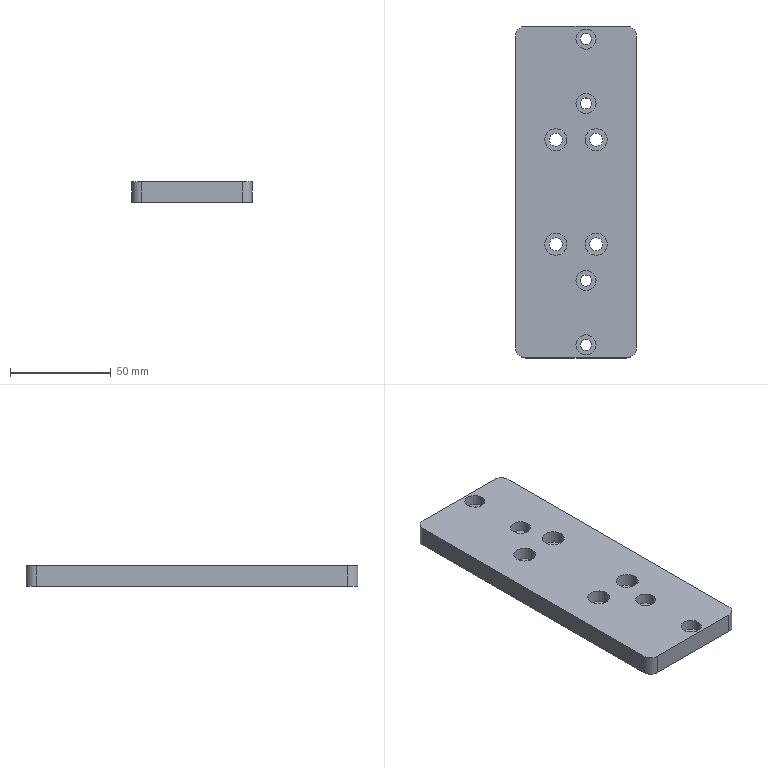Part | SolidWorks | features HoleWzd 2, Extrusion 1, Fillet 1 | 1 solid | 50 faces | box 60 x 165 x 10 mm | volume 93726 mm3 | cylinder 36 | plane 14 | commonest cylinder face diameters 10 x12 5.5 x8 6.6 x8 11 x8
STEP:
#1=CARTESIAN_POINT('',(-0.05704,76.,4.6));
#2=VERTEX_POINT('',#1);
#3=CARTESIAN_POINT('',(9.943,76.,4.6));
#4=VERTEX_POINT('',#3);
#5=CARTESIAN_POINT('',(4.943,76.,4.6));
#6=DIRECTION('',(0.,0.,1.));
#7=DIRECTION('',(1.,0.,0.));
#8=AXIS2_PLACEMENT_3D('',#5,#6,#7);
#9=CIRCLE('',#8,5.);
#10=EDGE_CURVE('',#2,#4,#9,.T.);
#11=ORIENTED_EDGE('',*,*,#10,.F.);
#12=CARTESIAN_POINT('',(-0.05704,76.,10.));
#13=VERTEX_POINT('',#12);
#14=CARTESIAN_POINT('',(-0.05704,76.,10.));
#15=DIRECTION('',(0.,0.,1.));
#16=VECTOR('',#15,1000.);
#17=LINE('',#14,#16);
#18=EDGE_CURVE('',#2,#13,#17,.T.);
#19=ORIENTED_EDGE('',*,*,#18,.T.);
#20=CARTESIAN_POINT('',(9.943,76.,10.));
#21=VERTEX_POINT('',#20);
#22=CARTESIAN_POINT('',(4.943,76.,10.));
#23=DIRECTION('',(0.,0.,1.));
#24=DIRECTION('',(1.,0.,0.));
#25=AXIS2_PLACEMENT_3D('',#22,#23,#24);
#26=CIRCLE('',#25,5.);
#27=EDGE_CURVE('',#13,#21,#26,.T.);
#28=ORIENTED_EDGE('',*,*,#27,.T.);
#29=CARTESIAN_POINT('',(9.943,76.,10.));
#30=DIRECTION('',(0.,0.,1.));
#31=VECTOR('',#30,1000.);
#32=LINE('',#29,#31);
#33=EDGE_CURVE('',#4,#21,#32,.T.);
#34=ORIENTED_EDGE('',*,*,#33,.F.);
#35=EDGE_LOOP('',(#11,#19,#28,#34));
#36=FACE_OUTER_BOUND('',#35,.T.);
#37=CARTESIAN_POINT('',(4.943,76.,10.));
#38=DIRECTION('',(0.,0.,1.));
#39=DIRECTION('',(1.,0.,0.));
#40=AXIS2_PLACEMENT_3D('',#37,#38,#39);
#41=CYLINDRICAL_SURFACE('',#40,5.);
#42=ADVANCED_FACE('',(#36),#41,.F.);
#43=CARTESIAN_POINT('',(2.193,76.,0.));
#44=VERTEX_POINT('',#43);
#45=CARTESIAN_POINT('',(7.693,76.,0.));
#46=VERTEX_POINT('',#45);
#47=CARTESIAN_POINT('',(4.943,76.,0.));
#48=DIRECTION('',(0.,0.,1.));
#49=DIRECTION('',(1.,0.,0.));
#50=AXIS2_PLACEMENT_3D('',#47,#48,#49);
#51=CIRCLE('',#50,2.75);
#52=EDGE_CURVE('',#44,#46,#51,.T.);
#53=ORIENTED_EDGE('',*,*,#52,.F.);
#54=CARTESIAN_POINT('',(2.193,76.,4.6));
#55=VERTEX_POINT('',#54);
#56=CARTESIAN_POINT('',(2.193,76.,10.));
#57=DIRECTION('',(0.,0.,1.));
#58=VECTOR('',#57,1000.);
#59=LINE('',#56,#58);
#60=EDGE_CURVE('',#44,#55,#59,.T.);
#61=ORIENTED_EDGE('',*,*,#60,.T.);
#62=CARTESIAN_POINT('',(7.693,76.,4.6));
#63=VERTEX_POINT('',#62);
#64=CARTESIAN_POINT('',(4.943,76.,4.6));
#65=DIRECTION('',(0.,0.,1.));
#66=DIRECTION('',(1.,0.,0.));
#67=AXIS2_PLACEMENT_3D('',#64,#65,#66);
#68=CIRCLE('',#67,2.75);
#69=EDGE_CURVE('',#55,#63,#68,.T.);
#70=ORIENTED_EDGE('',*,*,#69,.T.);
#71=CARTESIAN_POINT('',(7.693,76.,10.));
#72=DIRECTION('',(0.,0.,1.));
#73=VECTOR('',#72,1000.);
#74=LINE('',#71,#73);
#75=EDGE_CURVE('',#46,#63,#74,.T.);
#76=ORIENTED_EDGE('',*,*,#75,.F.);
#77=EDGE_LOOP('',(#53,#61,#70,#76));
#78=FACE_OUTER_BOUND('',#77,.T.);
#79=CARTESIAN_POINT('',(4.943,76.,10.));
#80=DIRECTION('',(0.,0.,1.));
#81=DIRECTION('',(1.,0.,0.));
#82=AXIS2_PLACEMENT_3D('',#79,#80,#81);
#83=CYLINDRICAL_SURFACE('',#82,2.75);
#84=ADVANCED_FACE('',(#78),#83,.F.);
#85=CARTESIAN_POINT('',(-0.05704,44.,4.6));
#86=VERTEX_POINT('',#85);
#87=CARTESIAN_POINT('',(9.943,44.,4.6));
#88=VERTEX_POINT('',#87);
#89=CARTESIAN_POINT('',(4.943,44.,4.6));
#90=DIRECTION('',(0.,0.,1.));
#91=DIRECTION('',(1.,0.,0.));
#92=AXIS2_PLACEMENT_3D('',#89,#90,#91);
#93=CIRCLE('',#92,5.);
#94=EDGE_CURVE('',#86,#88,#93,.T.);
#95=ORIENTED_EDGE('',*,*,#94,.F.);
#96=CARTESIAN_POINT('',(-0.05704,44.,10.));
#97=VERTEX_POINT('',#96);
#98=CARTESIAN_POINT('',(-0.05704,44.,10.));
#99=DIRECTION('',(0.,0.,1.));
#100=VECTOR('',#99,1000.);
#101=LINE('',#98,#100);
#102=EDGE_CURVE('',#86,#97,#101,.T.);
#103=ORIENTED_EDGE('',*,*,#102,.T.);
#104=CARTESIAN_POINT('',(9.943,44.,10.));
#105=VERTEX_POINT('',#104);
#106=CARTESIAN_POINT('',(4.943,44.,10.));
#107=DIRECTION('',(0.,0.,1.));
#108=DIRECTION('',(1.,0.,0.));
#109=AXIS2_PLACEMENT_3D('',#106,#107,#108);
#110=CIRCLE('',#109,5.);
#111=EDGE_CURVE('',#97,#105,#110,.T.);
#112=ORIENTED_EDGE('',*,*,#111,.T.);
#113=CARTESIAN_POINT('',(9.943,44.,10.));
#114=DIRECTION('',(0.,0.,1.));
#115=VECTOR('',#114,1000.);
#116=LINE('',#113,#115);
#117=EDGE_CURVE('',#88,#105,#116,.T.);
#118=ORIENTED_EDGE('',*,*,#117,.F.);
#119=EDGE_LOOP('',(#95,#103,#112,#118));
#120=FACE_OUTER_BOUND('',#119,.T.);
#121=CARTESIAN_POINT('',(4.943,44.,10.));
#122=DIRECTION('',(0.,0.,1.));
#123=DIRECTION('',(1.,0.,0.));
#124=AXIS2_PLACEMENT_3D('',#121,#122,#123);
#125=CYLINDRICAL_SURFACE('',#124,5.);
#126=ADVANCED_FACE('',(#120),#125,.F.);
#127=CARTESIAN_POINT('',(2.193,44.,0.));
#128=VERTEX_POINT('',#127);
#129=CARTESIAN_POINT('',(7.693,44.,0.));
#130=VERTEX_POINT('',#129);
#131=CARTESIAN_POINT('',(4.943,44.,0.));
#132=DIRECTION('',(0.,0.,1.));
#133=DIRECTION('',(1.,0.,0.));
#134=AXIS2_PLACEMENT_3D('',#131,#132,#133);
#135=CIRCLE('',#134,2.75);
#136=EDGE_CURVE('',#128,#130,#135,.T.);
#137=ORIENTED_EDGE('',*,*,#136,.F.);
#138=CARTESIAN_POINT('',(2.193,44.,4.6));
#139=VERTEX_POINT('',#138);
#140=CARTESIAN_POINT('',(2.193,44.,10.));
#141=DIRECTION('',(0.,0.,1.));
#142=VECTOR('',#141,1000.);
#143=LINE('',#140,#142);
#144=EDGE_CURVE('',#128,#139,#143,.T.);
#145=ORIENTED_EDGE('',*,*,#144,.T.);
#146=CARTESIAN_POINT('',(7.693,44.,4.6));
#147=VERTEX_POINT('',#146);
#148=CARTESIAN_POINT('',(4.943,44.,4.6));
#149=DIRECTION('',(0.,0.,1.));
#150=DIRECTION('',(1.,0.,0.));
#151=AXIS2_PLACEMENT_3D('',#148,#149,#150);
#152=CIRCLE('',#151,2.75);
#153=EDGE_CURVE('',#139,#147,#152,.T.);
#154=ORIENTED_EDGE('',*,*,#153,.T.);
#155=CARTESIAN_POINT('',(7.693,44.,10.));
#156=DIRECTION('',(0.,0.,1.));
#157=VECTOR('',#156,1000.);
#158=LINE('',#155,#157);
#159=EDGE_CURVE('',#130,#147,#158,.T.);
#160=ORIENTED_EDGE('',*,*,#159,.F.);
#161=EDGE_LOOP('',(#137,#145,#154,#160));
#162=FACE_OUTER_BOUND('',#161,.T.);
#163=CARTESIAN_POINT('',(4.943,44.,10.));
#164=DIRECTION('',(0.,0.,1.));
#165=DIRECTION('',(1.,0.,0.));
#166=AXIS2_PLACEMENT_3D('',#163,#164,#165);
#167=CYLINDRICAL_SURFACE('',#166,2.75);
#168=ADVANCED_FACE('',(#162),#167,.F.);
#169=CARTESIAN_POINT('',(-0.05704,-44.,4.6));
#170=VERTEX_POINT('',#169);
#171=CARTESIAN_POINT('',(9.943,-44.,4.6));
#172=VERTEX_POINT('',#171);
#173=CARTESIAN_POINT('',(4.943,-44.,4.6));
#174=DIRECTION('',(0.,0.,1.));
#175=DIRECTION('',(1.,0.,0.));
#176=AXIS2_PLACEMENT_3D('',#173,#174,#175);
#177=CIRCLE('',#176,5.);
#178=EDGE_CURVE('',#170,#172,#177,.T.);
#179=ORIENTED_EDGE('',*,*,#178,.F.);
#180=CARTESIAN_POINT('',(-0.05704,-44.,10.));
#181=VERTEX_POINT('',#180);
#182=CARTESIAN_POINT('',(-0.05704,-44.,10.));
#183=DIRECTION('',(0.,0.,1.));
#184=VECTOR('',#183,1000.);
#185=LINE('',#182,#184);
#186=EDGE_CURVE('',#170,#181,#185,.T.);
#187=ORIENTED_EDGE('',*,*,#186,.T.);
#188=CARTESIAN_POINT('',(9.943,-44.,10.));
#189=VERTEX_POINT('',#188);
#190=CARTESIAN_POINT('',(4.943,-44.,10.));
#191=DIRECTION('',(0.,0.,1.));
#192=DIRECTION('',(1.,0.,0.));
#193=AXIS2_PLACEMENT_3D('',#190,#191,#192);
#194=CIRCLE('',#193,5.);
#195=EDGE_CURVE('',#181,#189,#194,.T.);
#196=ORIENTED_EDGE('',*,*,#195,.T.);
#197=CARTESIAN_POINT('',(9.943,-44.,10.));
#198=DIRECTION('',(0.,0.,1.));
#199=VECTOR('',#198,1000.);
#200=LINE('',#197,#199);
#201=EDGE_CURVE('',#172,#189,#200,.T.);
#202=ORIENTED_EDGE('',*,*,#201,.F.);
#203=EDGE_LOOP('',(#179,#187,#196,#202));
#204=FACE_OUTER_BOUND('',#203,.T.);
#205=CARTESIAN_POINT('',(4.943,-44.,10.));
#206=DIRECTION('',(0.,0.,1.));
#207=DIRECTION('',(1.,0.,0.));
#208=AXIS2_PLACEMENT_3D('',#205,#206,#207);
#209=CYLINDRICAL_SURFACE('',#208,5.);
#210=ADVANCED_FACE('',(#204),#209,.F.);
#211=CARTESIAN_POINT('',(2.193,-44.,0.));
#212=VERTEX_POINT('',#211);
#213=CARTESIAN_POINT('',(7.693,-44.,0.));
#214=VERTEX_POINT('',#213);
#215=CARTESIAN_POINT('',(4.943,-44.,0.));
#216=DIRECTION('',(0.,0.,1.));
#217=DIRECTION('',(1.,0.,0.));
#218=AXIS2_PLACEMENT_3D('',#215,#216,#217);
#219=CIRCLE('',#218,2.75);
#220=EDGE_CURVE('',#212,#214,#219,.T.);
#221=ORIENTED_EDGE('',*,*,#220,.F.);
#222=CARTESIAN_POINT('',(2.193,-44.,4.6));
#223=VERTEX_POINT('',#222);
#224=CARTESIAN_POINT('',(2.193,-44.,10.));
#225=DIRECTION('',(0.,0.,1.));
#226=VECTOR('',#225,1000.);
#227=LINE('',#224,#226);
#228=EDGE_CURVE('',#212,#223,#227,.T.);
#229=ORIENTED_EDGE('',*,*,#228,.T.);
#230=CARTESIAN_POINT('',(7.693,-44.,4.6));
#231=VERTEX_POINT('',#230);
#232=CARTESIAN_POINT('',(4.943,-44.,4.6));
#233=DIRECTION('',(0.,0.,1.));
#234=DIRECTION('',(1.,0.,0.));
#235=AXIS2_PLACEMENT_3D('',#232,#233,#234);
#236=CIRCLE('',#235,2.75);
#237=EDGE_CURVE('',#223,#231,#236,.T.);
#238=ORIENTED_EDGE('',*,*,#237,.T.);
#239=CARTESIAN_POINT('',(7.693,-44.,10.));
#240=DIRECTION('',(0.,0.,1.));
#241=VECTOR('',#240,1000.);
#242=LINE('',#239,#241);
#243=EDGE_CURVE('',#214,#231,#242,.T.);
#244=ORIENTED_EDGE('',*,*,#243,.F.);
#245=EDGE_LOOP('',(#221,#229,#238,#244));
#246=FACE_OUTER_BOUND('',#245,.T.);
#247=CARTESIAN_POINT('',(4.943,-44.,10.));
#248=DIRECTION('',(0.,0.,1.));
#249=DIRECTION('',(1.,0.,0.));
#250=AXIS2_PLACEMENT_3D('',#247,#248,#249);
#251=CYLINDRICAL_SURFACE('',#250,2.75);
#252=ADVANCED_FACE('',(#246),#251,.F.);
#253=CARTESIAN_POINT('',(-0.05704,-76.,4.6));
#254=VERTEX_POINT('',#253);
#255=CARTESIAN_POINT('',(9.943,-76.,4.6));
#256=VERTEX_POINT('',#255);
#257=CARTESIAN_POINT('',(4.943,-76.,4.6));
#258=DIRECTION('',(0.,0.,1.));
#259=DIRECTION('',(1.,0.,0.));
#260=AXIS2_PLACEMENT_3D('',#257,#258,#259);
#261=CIRCLE('',#260,5.);
#262=EDGE_CURVE('',#254,#256,#261,.T.);
#263=ORIENTED_EDGE('',*,*,#262,.F.);
#264=CARTESIAN_POINT('',(-0.05704,-76.,10.));
#265=VERTEX_POINT('',#264);
#266=CARTESIAN_POINT('',(-0.05704,-76.,10.));
#267=DIRECTION('',(0.,0.,1.));
#268=VECTOR('',#267,1000.);
#269=LINE('',#266,#268);
#270=EDGE_CURVE('',#254,#265,#269,.T.);
#271=ORIENTED_EDGE('',*,*,#270,.T.);
#272=CARTESIAN_POINT('',(9.943,-76.,10.));
#273=VERTEX_POINT('',#272);
#274=CARTESIAN_POINT('',(4.943,-76.,10.));
#275=DIRECTION('',(0.,0.,1.));
#276=DIRECTION('',(1.,0.,0.));
#277=AXIS2_PLACEMENT_3D('',#274,#275,#276);
#278=CIRCLE('',#277,5.);
#279=EDGE_CURVE('',#265,#273,#278,.T.);
#280=ORIENTED_EDGE('',*,*,#279,.T.);
#281=CARTESIAN_POINT('',(9.943,-76.,10.));
#282=DIRECTION('',(0.,0.,1.));
#283=VECTOR('',#282,1000.);
#284=LINE('',#281,#283);
#285=EDGE_CURVE('',#256,#273,#284,.T.);
#286=ORIENTED_EDGE('',*,*,#285,.F.);
#287=EDGE_LOOP('',(#263,#271,#280,#286));
#288=FACE_OUTER_BOUND('',#287,.T.);
#289=CARTESIAN_POINT('',(4.943,-76.,10.));
#290=DIRECTION('',(0.,0.,1.));
#291=DIRECTION('',(1.,0.,0.));
#292=AXIS2_PLACEMENT_3D('',#289,#290,#291);
#293=CYLINDRICAL_SURFACE('',#292,5.);
#294=ADVANCED_FACE('',(#288),#293,.F.);
#295=CARTESIAN_POINT('',(2.193,-76.,0.));
#296=VERTEX_POINT('',#295);
#297=CARTESIAN_POINT('',(7.693,-76.,0.));
#298=VERTEX_POINT('',#297);
#299=CARTESIAN_POINT('',(4.943,-76.,0.));
#300=DIRECTION('',(0.,0.,1.));
#301=DIRECTION('',(1.,0.,0.));
#302=AXIS2_PLACEMENT_3D('',#299,#300,#301);
#303=CIRCLE('',#302,2.75);
#304=EDGE_CURVE('',#296,#298,#303,.T.);
#305=ORIENTED_EDGE('',*,*,#304,.F.);
#306=CARTESIAN_POINT('',(2.193,-76.,4.6));
#307=VERTEX_POINT('',#306);
#308=CARTESIAN_POINT('',(2.193,-76.,10.));
#309=DIRECTION('',(0.,0.,1.));
#310=VECTOR('',#309,1000.);
#311=LINE('',#308,#310);
#312=EDGE_CURVE('',#296,#307,#311,.T.);
#313=ORIENTED_EDGE('',*,*,#312,.T.);
#314=CARTESIAN_POINT('',(7.693,-76.,4.6));
#315=VERTEX_POINT('',#314);
#316=CARTESIAN_POINT('',(4.943,-76.,4.6));
#317=DIRECTION('',(0.,0.,1.));
#318=DIRECTION('',(1.,0.,0.));
#319=AXIS2_PLACEMENT_3D('',#316,#317,#318);
#320=CIRCLE('',#319,2.75);
#321=EDGE_CURVE('',#307,#315,#320,.T.);
#322=ORIENTED_EDGE('',*,*,#321,.T.);
#323=CARTESIAN_POINT('',(7.693,-76.,10.));
#324=DIRECTION('',(0.,0.,1.));
#325=VECTOR('',#324,1000.);
#326=LINE('',#323,#325);
#327=EDGE_CURVE('',#298,#315,#326,.T.);
#328=ORIENTED_EDGE('',*,*,#327,.F.);
#329=EDGE_LOOP('',(#305,#313,#322,#328));
#330=FACE_OUTER_BOUND('',#329,.T.);
#331=CARTESIAN_POINT('',(4.943,-76.,10.));
#332=DIRECTION('',(0.,0.,1.));
#333=DIRECTION('',(1.,0.,0.));
#334=AXIS2_PLACEMENT_3D('',#331,#332,#333);
#335=CYLINDRICAL_SURFACE('',#334,2.75);
#336=ADVANCED_FACE('',(#330),#335,.F.);
#337=CARTESIAN_POINT('',(-15.5,26.,3.6));
#338=VERTEX_POINT('',#337);
#339=CARTESIAN_POINT('',(-4.5,26.,3.6));
#340=VERTEX_POINT('',#339);
#341=CARTESIAN_POINT('',(-10.,26.,3.6));
#342=DIRECTION('',(0.,0.,1.));
#343=DIRECTION('',(1.,0.,0.));
#344=AXIS2_PLACEMENT_3D('',#341,#342,#343);
#345=CIRCLE('',#344,5.5);
#346=EDGE_CURVE('',#338,#340,#345,.T.);
#347=ORIENTED_EDGE('',*,*,#346,.F.);
#348=CARTESIAN_POINT('',(-15.5,26.,10.));
#349=VERTEX_POINT('',#348);
#350=CARTESIAN_POINT('',(-15.5,26.,10.));
#351=DIRECTION('',(0.,0.,1.));
#352=VECTOR('',#351,1000.);
#353=LINE('',#350,#352);
#354=EDGE_CURVE('',#338,#349,#353,.T.);
#355=ORIENTED_EDGE('',*,*,#354,.T.);
#356=CARTESIAN_POINT('',(-4.5,26.,10.));
#357=VERTEX_POINT('',#356);
#358=CARTESIAN_POINT('',(-10.,26.,10.));
#359=DIRECTION('',(0.,0.,1.));
#360=DIRECTION('',(1.,0.,0.));
#361=AXIS2_PLACEMENT_3D('',#358,#359,#360);
#362=CIRCLE('',#361,5.5);
#363=EDGE_CURVE('',#349,#357,#362,.T.);
#364=ORIENTED_EDGE('',*,*,#363,.T.);
#365=CARTESIAN_POINT('',(-4.5,26.,10.));
#366=DIRECTION('',(0.,0.,1.));
#367=VECTOR('',#366,1000.);
#368=LINE('',#365,#367);
#369=EDGE_CURVE('',#340,#357,#368,.T.);
#370=ORIENTED_EDGE('',*,*,#369,.F.);
#371=EDGE_LOOP('',(#347,#355,#364,#370));
#372=FACE_OUTER_BOUND('',#371,.T.);
#373=CARTESIAN_POINT('',(-10.,26.,10.));
#374=DIRECTION('',(0.,0.,1.));
#375=DIRECTION('',(1.,0.,0.));
#376=AXIS2_PLACEMENT_3D('',#373,#374,#375);
#377=CYLINDRICAL_SURFACE('',#376,5.5);
#378=ADVANCED_FACE('',(#372),#377,.F.);
#379=CARTESIAN_POINT('',(-13.3,26.,0.));
#380=VERTEX_POINT('',#379);
#381=CARTESIAN_POINT('',(-6.7,26.,0.));
#382=VERTEX_POINT('',#381);
#383=CARTESIAN_POINT('',(-10.,26.,0.));
#384=DIRECTION('',(0.,0.,1.));
#385=DIRECTION('',(1.,0.,0.));
#386=AXIS2_PLACEMENT_3D('',#383,#384,#385);
#387=CIRCLE('',#386,3.3);
#388=EDGE_CURVE('',#380,#382,#387,.T.);
#389=ORIENTED_EDGE('',*,*,#388,.F.);
#390=CARTESIAN_POINT('',(-13.3,26.,3.6));
#391=VERTEX_POINT('',#390);
#392=CARTESIAN_POINT('',(-13.3,26.,10.));
#393=DIRECTION('',(0.,0.,1.));
#394=VECTOR('',#393,1000.);
#395=LINE('',#392,#394);
#396=EDGE_CURVE('',#380,#391,#395,.T.);
#397=ORIENTED_EDGE('',*,*,#396,.T.);
#398=CARTESIAN_POINT('',(-6.7,26.,3.6));
#399=VERTEX_POINT('',#398);
#400=CARTESIAN_POINT('',(-10.,26.,3.6));
#401=DIRECTION('',(0.,0.,1.));
#402=DIRECTION('',(1.,0.,0.));
#403=AXIS2_PLACEMENT_3D('',#400,#401,#402);
#404=CIRCLE('',#403,3.3);
#405=EDGE_CURVE('',#391,#399,#404,.T.);
#406=ORIENTED_EDGE('',*,*,#405,.T.);
#407=CARTESIAN_POINT('',(-6.7,26.,10.));
#408=DIRECTION('',(0.,0.,1.));
#409=VECTOR('',#408,1000.);
#410=LINE('',#407,#409);
#411=EDGE_CURVE('',#382,#399,#410,.T.);
#412=ORIENTED_EDGE('',*,*,#411,.F.);
#413=EDGE_LOOP('',(#389,#397,#406,#412));
#414=FACE_OUTER_BOUND('',#413,.T.);
#415=CARTESIAN_POINT('',(-10.,26.,10.));
#416=DIRECTION('',(0.,0.,1.));
#417=DIRECTION('',(1.,0.,0.));
#418=AXIS2_PLACEMENT_3D('',#415,#416,#417);
#419=CYLINDRICAL_SURFACE('',#418,3.3);
#420=ADVANCED_FACE('',(#414),#419,.F.);
#421=CARTESIAN_POINT('',(4.5,26.,3.6));
#422=VERTEX_POINT('',#421);
#423=CARTESIAN_POINT('',(15.5,26.,3.6));
#424=VERTEX_POINT('',#423);
#425=CARTESIAN_POINT('',(10.,26.,3.6));
#426=DIRECTION('',(0.,0.,1.));
#427=DIRECTION('',(1.,0.,0.));
#428=AXIS2_PLACEMENT_3D('',#425,#426,#427);
#429=CIRCLE('',#428,5.5);
#430=EDGE_CURVE('',#422,#424,#429,.T.);
#431=ORIENTED_EDGE('',*,*,#430,.F.);
#432=CARTESIAN_POINT('',(4.5,26.,10.));
#433=VERTEX_POINT('',#432);
#434=CARTESIAN_POINT('',(4.5,26.,10.));
#435=DIRECTION('',(0.,0.,1.));
#436=VECTOR('',#435,1000.);
#437=LINE('',#434,#436);
#438=EDGE_CURVE('',#422,#433,#437,.T.);
#439=ORIENTED_EDGE('',*,*,#438,.T.);
#440=CARTESIAN_POINT('',(15.5,26.,10.));
#441=VERTEX_POINT('',#440);
#442=CARTESIAN_POINT('',(10.,26.,10.));
#443=DIRECTION('',(0.,0.,1.));
#444=DIRECTION('',(1.,0.,0.));
#445=AXIS2_PLACEMENT_3D('',#442,#443,#444);
#446=CIRCLE('',#445,5.5);
#447=EDGE_CURVE('',#433,#441,#446,.T.);
#448=ORIENTED_EDGE('',*,*,#447,.T.);
#449=CARTESIAN_POINT('',(15.5,26.,10.));
#450=DIRECTION('',(0.,0.,1.));
#451=VECTOR('',#450,1000.);
#452=LINE('',#449,#451);
#453=EDGE_CURVE('',#424,#441,#452,.T.);
#454=ORIENTED_EDGE('',*,*,#453,.F.);
#455=EDGE_LOOP('',(#431,#439,#448,#454));
#456=FACE_OUTER_BOUND('',#455,.T.);
#457=CARTESIAN_POINT('',(10.,26.,10.));
#458=DIRECTION('',(0.,0.,1.));
#459=DIRECTION('',(1.,0.,0.));
#460=AXIS2_PLACEMENT_3D('',#457,#458,#459);
#461=CYLINDRICAL_SURFACE('',#460,5.5);
#462=ADVANCED_FACE('',(#456),#461,.F.);
#463=CARTESIAN_POINT('',(6.7,26.,0.));
#464=VERTEX_POINT('',#463);
#465=CARTESIAN_POINT('',(13.3,26.,0.));
#466=VERTEX_POINT('',#465);
#467=CARTESIAN_POINT('',(10.,26.,0.));
#468=DIRECTION('',(0.,0.,1.));
#469=DIRECTION('',(1.,0.,0.));
#470=AXIS2_PLACEMENT_3D('',#467,#468,#469);
#471=CIRCLE('',#470,3.3);
#472=EDGE_CURVE('',#464,#466,#471,.T.);
#473=ORIENTED_EDGE('',*,*,#472,.F.);
#474=CARTESIAN_POINT('',(6.7,26.,3.6));
#475=VERTEX_POINT('',#474);
#476=CARTESIAN_POINT('',(6.7,26.,10.));
#477=DIRECTION('',(0.,0.,1.));
#478=VECTOR('',#477,1000.);
#479=LINE('',#476,#478);
#480=EDGE_CURVE('',#464,#475,#479,.T.);
#481=ORIENTED_EDGE('',*,*,#480,.T.);
#482=CARTESIAN_POINT('',(13.3,26.,3.6));
#483=VERTEX_POINT('',#482);
#484=CARTESIAN_POINT('',(10.,26.,3.6));
#485=DIRECTION('',(0.,0.,1.));
#486=DIRECTION('',(1.,0.,0.));
#487=AXIS2_PLACEMENT_3D('',#484,#485,#486);
#488=CIRCLE('',#487,3.3);
#489=EDGE_CURVE('',#475,#483,#488,.T.);
#490=ORIENTED_EDGE('',*,*,#489,.T.);
#491=CARTESIAN_POINT('',(13.3,26.,10.));
#492=DIRECTION('',(0.,0.,1.));
#493=VECTOR('',#492,1000.);
#494=LINE('',#491,#493);
#495=EDGE_CURVE('',#466,#483,#494,.T.);
#496=ORIENTED_EDGE('',*,*,#495,.F.);
#497=EDGE_LOOP('',(#473,#481,#490,#496));
#498=FACE_OUTER_BOUND('',#497,.T.);
#499=CARTESIAN_POINT('',(10.,26.,10.));
#500=DIRECTION('',(0.,0.,1.));
#501=DIRECTION('',(1.,0.,0.));
#502=AXIS2_PLACEMENT_3D('',#499,#500,#501);
#503=CYLINDRICAL_SURFACE('',#502,3.3);
#504=ADVANCED_FACE('',(#498),#503,.F.);
#505=CARTESIAN_POINT('',(4.5,-26.,3.6));
#506=VERTEX_POINT('',#505);
#507=CARTESIAN_POINT('',(15.5,-26.,3.6));
#508=VERTEX_POINT('',#507);
#509=CARTESIAN_POINT('',(10.,-26.,3.6));
#510=DIRECTION('',(0.,0.,1.));
#511=DIRECTION('',(1.,0.,0.));
#512=AXIS2_PLACEMENT_3D('',#509,#510,#511);
#513=CIRCLE('',#512,5.5);
#514=EDGE_CURVE('',#506,#508,#513,.T.);
#515=ORIENTED_EDGE('',*,*,#514,.F.);
#516=CARTESIAN_POINT('',(4.5,-26.,10.));
#517=VERTEX_POINT('',#516);
#518=CARTESIAN_POINT('',(4.5,-26.,10.));
#519=DIRECTION('',(0.,0.,1.));
#520=VECTOR('',#519,1000.);
#521=LINE('',#518,#520);
#522=EDGE_CURVE('',#506,#517,#521,.T.);
#523=ORIENTED_EDGE('',*,*,#522,.T.);
#524=CARTESIAN_POINT('',(15.5,-26.,10.));
#525=VERTEX_POINT('',#524);
#526=CARTESIAN_POINT('',(10.,-26.,10.));
#527=DIRECTION('',(0.,0.,1.));
#528=DIRECTION('',(1.,0.,0.));
#529=AXIS2_PLACEMENT_3D('',#526,#527,#528);
#530=CIRCLE('',#529,5.5);
#531=EDGE_CURVE('',#517,#525,#530,.T.);
#532=ORIENTED_EDGE('',*,*,#531,.T.);
#533=CARTESIAN_POINT('',(15.5,-26.,10.));
#534=DIRECTION('',(0.,0.,1.));
#535=VECTOR('',#534,1000.);
#536=LINE('',#533,#535);
#537=EDGE_CURVE('',#508,#525,#536,.T.);
#538=ORIENTED_EDGE('',*,*,#537,.F.);
#539=EDGE_LOOP('',(#515,#523,#532,#538));
#540=FACE_OUTER_BOUND('',#539,.T.);
#541=CARTESIAN_POINT('',(10.,-26.,10.));
#542=DIRECTION('',(0.,0.,1.));
#543=DIRECTION('',(1.,0.,0.));
#544=AXIS2_PLACEMENT_3D('',#541,#542,#543);
#545=CYLINDRICAL_SURFACE('',#544,5.5);
#546=ADVANCED_FACE('',(#540),#545,.F.);
#547=CARTESIAN_POINT('',(6.7,-26.,0.));
#548=VERTEX_POINT('',#547);
#549=CARTESIAN_POINT('',(13.3,-26.,0.));
#550=VERTEX_POINT('',#549);
#551=CARTESIAN_POINT('',(10.,-26.,0.));
#552=DIRECTION('',(0.,0.,1.));
#553=DIRECTION('',(1.,0.,0.));
#554=AXIS2_PLACEMENT_3D('',#551,#552,#553);
#555=CIRCLE('',#554,3.3);
#556=EDGE_CURVE('',#548,#550,#555,.T.);
#557=ORIENTED_EDGE('',*,*,#556,.F.);
#558=CARTESIAN_POINT('',(6.7,-26.,3.6));
#559=VERTEX_POINT('',#558);
#560=CARTESIAN_POINT('',(6.7,-26.,10.));
#561=DIRECTION('',(0.,0.,1.));
#562=VECTOR('',#561,1000.);
#563=LINE('',#560,#562);
#564=EDGE_CURVE('',#548,#559,#563,.T.);
#565=ORIENTED_EDGE('',*,*,#564,.T.);
#566=CARTESIAN_POINT('',(13.3,-26.,3.6));
#567=VERTEX_POINT('',#566);
#568=CARTESIAN_POINT('',(10.,-26.,3.6));
#569=DIRECTION('',(0.,0.,1.));
#570=DIRECTION('',(1.,0.,0.));
#571=AXIS2_PLACEMENT_3D('',#568,#569,#570);
#572=CIRCLE('',#571,3.3);
#573=EDGE_CURVE('',#559,#567,#572,.T.);
#574=ORIENTED_EDGE('',*,*,#573,.T.);
#575=CARTESIAN_POINT('',(13.3,-26.,10.));
#576=DIRECTION('',(0.,0.,1.));
#577=VECTOR('',#576,1000.);
#578=LINE('',#575,#577);
#579=EDGE_CURVE('',#550,#567,#578,.T.);
#580=ORIENTED_EDGE('',*,*,#579,.F.);
#581=EDGE_LOOP('',(#557,#565,#574,#580));
#582=FACE_OUTER_BOUND('',#581,.T.);
#583=CARTESIAN_POINT('',(10.,-26.,10.));
#584=DIRECTION('',(0.,0.,1.));
#585=DIRECTION('',(1.,0.,0.));
#586=AXIS2_PLACEMENT_3D('',#583,#584,#585);
#587=CYLINDRICAL_SURFACE('',#586,3.3);
#588=ADVANCED_FACE('',(#582),#587,.F.);
#589=CARTESIAN_POINT('',(-15.5,-26.,3.6));
#590=VERTEX_POINT('',#589);
#591=CARTESIAN_POINT('',(-4.5,-26.,3.6));
#592=VERTEX_POINT('',#591);
#593=CARTESIAN_POINT('',(-10.,-26.,3.6));
#594=DIRECTION('',(0.,0.,1.));
#595=DIRECTION('',(1.,0.,0.));
#596=AXIS2_PLACEMENT_3D('',#593,#594,#595);
#597=CIRCLE('',#596,5.5);
#598=EDGE_CURVE('',#590,#592,#597,.T.);
#599=ORIENTED_EDGE('',*,*,#598,.F.);
#600=CARTESIAN_POINT('',(-15.5,-26.,10.));
#601=VERTEX_POINT('',#600);
#602=CARTESIAN_POINT('',(-15.5,-26.,10.));
#603=DIRECTION('',(0.,0.,1.));
#604=VECTOR('',#603,1000.);
#605=LINE('',#602,#604);
#606=EDGE_CURVE('',#590,#601,#605,.T.);
#607=ORIENTED_EDGE('',*,*,#606,.T.);
#608=CARTESIAN_POINT('',(-4.5,-26.,10.));
#609=VERTEX_POINT('',#608);
#610=CARTESIAN_POINT('',(-10.,-26.,10.));
#611=DIRECTION('',(0.,0.,1.));
#612=DIRECTION('',(1.,0.,0.));
#613=AXIS2_PLACEMENT_3D('',#610,#611,#612);
#614=CIRCLE('',#613,5.5);
#615=EDGE_CURVE('',#601,#609,#614,.T.);
#616=ORIENTED_EDGE('',*,*,#615,.T.);
#617=CARTESIAN_POINT('',(-4.5,-26.,10.));
#618=DIRECTION('',(0.,0.,1.));
#619=VECTOR('',#618,1000.);
#620=LINE('',#617,#619);
#621=EDGE_CURVE('',#592,#609,#620,.T.);
#622=ORIENTED_EDGE('',*,*,#621,.F.);
#623=EDGE_LOOP('',(#599,#607,#616,#622));
#624=FACE_OUTER_BOUND('',#623,.T.);
#625=CARTESIAN_POINT('',(-10.,-26.,10.));
#626=DIRECTION('',(0.,0.,1.));
#627=DIRECTION('',(1.,0.,0.));
#628=AXIS2_PLACEMENT_3D('',#625,#626,#627);
#629=CYLINDRICAL_SURFACE('',#628,5.5);
#630=ADVANCED_FACE('',(#624),#629,.F.);
#631=CARTESIAN_POINT('',(-13.3,-26.,0.));
#632=VERTEX_POINT('',#631);
#633=CARTESIAN_POINT('',(-6.7,-26.,0.));
#634=VERTEX_POINT('',#633);
#635=CARTESIAN_POINT('',(-10.,-26.,0.));
#636=DIRECTION('',(0.,0.,1.));
#637=DIRECTION('',(1.,0.,0.));
#638=AXIS2_PLACEMENT_3D('',#635,#636,#637);
#639=CIRCLE('',#638,3.3);
#640=EDGE_CURVE('',#632,#634,#639,.T.);
#641=ORIENTED_EDGE('',*,*,#640,.F.);
#642=CARTESIAN_POINT('',(-13.3,-26.,3.6));
#643=VERTEX_POINT('',#642);
#644=CARTESIAN_POINT('',(-13.3,-26.,10.));
#645=DIRECTION('',(0.,0.,1.));
#646=VECTOR('',#645,1000.);
#647=LINE('',#644,#646);
#648=EDGE_CURVE('',#632,#643,#647,.T.);
#649=ORIENTED_EDGE('',*,*,#648,.T.);
#650=CARTESIAN_POINT('',(-6.7,-26.,3.6));
#651=VERTEX_POINT('',#650);
#652=CARTESIAN_POINT('',(-10.,-26.,3.6));
#653=DIRECTION('',(0.,0.,1.));
#654=DIRECTION('',(1.,0.,0.));
#655=AXIS2_PLACEMENT_3D('',#652,#653,#654);
#656=CIRCLE('',#655,3.3);
#657=EDGE_CURVE('',#643,#651,#656,.T.);
#658=ORIENTED_EDGE('',*,*,#657,.T.);
#659=CARTESIAN_POINT('',(-6.7,-26.,10.));
#660=DIRECTION('',(0.,0.,1.));
#661=VECTOR('',#660,1000.);
#662=LINE('',#659,#661);
#663=EDGE_CURVE('',#634,#651,#662,.T.);
#664=ORIENTED_EDGE('',*,*,#663,.F.);
#665=EDGE_LOOP('',(#641,#649,#658,#664));
#666=FACE_OUTER_BOUND('',#665,.T.);
#667=CARTESIAN_POINT('',(-10.,-26.,10.));
#668=DIRECTION('',(0.,0.,1.));
#669=DIRECTION('',(1.,0.,0.));
#670=AXIS2_PLACEMENT_3D('',#667,#668,#669);
#671=CYLINDRICAL_SURFACE('',#670,3.3);
#672=ADVANCED_FACE('',(#666),#671,.F.);
#673=CARTESIAN_POINT('',(30.,-77.5,0.));
#674=VERTEX_POINT('',#673);
#675=CARTESIAN_POINT('',(30.,77.5,0.));
#676=VERTEX_POINT('',#675);
#677=CARTESIAN_POINT('',(30.,-82.5,0.));
#678=DIRECTION('',(0.,1.,0.));
#679=VECTOR('',#678,1000.);
#680=LINE('',#677,#679);
#681=EDGE_CURVE('',#674,#676,#680,.T.);
#682=ORIENTED_EDGE('',*,*,#681,.T.);
#683=CARTESIAN_POINT('',(30.,77.5,10.));
#684=VERTEX_POINT('',#683);
#685=CARTESIAN_POINT('',(30.,77.5,10.));
#686=DIRECTION('',(0.,0.,1.));
#687=VECTOR('',#686,1000.);
#688=LINE('',#685,#687);
#689=EDGE_CURVE('',#676,#684,#688,.T.);
#690=ORIENTED_EDGE('',*,*,#689,.T.);
#691=CARTESIAN_POINT('',(30.,-77.5,10.));
#692=VERTEX_POINT('',#691);
#693=CARTESIAN_POINT('',(30.,-82.5,10.));
#694=DIRECTION('',(0.,1.,0.));
#695=VECTOR('',#694,1000.);
#696=LINE('',#693,#695);
#697=EDGE_CURVE('',#692,#684,#696,.T.);
#698=ORIENTED_EDGE('',*,*,#697,.F.);
#699=CARTESIAN_POINT('',(30.,-77.5,10.));
#700=DIRECTION('',(0.,0.,-1.));
#701=VECTOR('',#700,1000.);
#702=LINE('',#699,#701);
#703=EDGE_CURVE('',#692,#674,#702,.T.);
#704=ORIENTED_EDGE('',*,*,#703,.T.);
#705=EDGE_LOOP('',(#682,#690,#698,#704));
#706=FACE_OUTER_BOUND('',#705,.T.);
#707=CARTESIAN_POINT('',(30.,-82.5,10.));
#708=DIRECTION('',(-1.,0.,0.));
#709=DIRECTION('',(0.,0.,1.));
#710=AXIS2_PLACEMENT_3D('',#707,#708,#709);
#711=PLANE('',#710);
#712=ADVANCED_FACE('',(#706),#711,.F.);
#713=CARTESIAN_POINT('',(25.,82.5,0.));
#714=VERTEX_POINT('',#713);
#715=CARTESIAN_POINT('',(-25.,82.5,0.));
#716=VERTEX_POINT('',#715);
#717=CARTESIAN_POINT('',(-30.,82.5,0.));
#718=DIRECTION('',(-1.,0.,0.));
#719=VECTOR('',#718,1000.);
#720=LINE('',#717,#719);
#721=EDGE_CURVE('',#714,#716,#720,.T.);
#722=ORIENTED_EDGE('',*,*,#721,.T.);
#723=CARTESIAN_POINT('',(-25.,82.5,10.));
#724=VERTEX_POINT('',#723);
#725=CARTESIAN_POINT('',(-25.,82.5,10.));
#726=DIRECTION('',(0.,0.,1.));
#727=VECTOR('',#726,1000.);
#728=LINE('',#725,#727);
#729=EDGE_CURVE('',#716,#724,#728,.T.);
#730=ORIENTED_EDGE('',*,*,#729,.T.);
#731=CARTESIAN_POINT('',(25.,82.5,10.));
#732=VERTEX_POINT('',#731);
#733=CARTESIAN_POINT('',(-30.,82.5,10.));
#734=DIRECTION('',(-1.,0.,0.));
#735=VECTOR('',#734,1000.);
#736=LINE('',#733,#735);
#737=EDGE_CURVE('',#732,#724,#736,.T.);
#738=ORIENTED_EDGE('',*,*,#737,.F.);
#739=CARTESIAN_POINT('',(25.,82.5,10.));
#740=DIRECTION('',(0.,0.,-1.));
#741=VECTOR('',#740,1000.);
#742=LINE('',#739,#741);
#743=EDGE_CURVE('',#732,#714,#742,.T.);
#744=ORIENTED_EDGE('',*,*,#743,.T.);
#745=EDGE_LOOP('',(#722,#730,#738,#744));
#746=FACE_OUTER_BOUND('',#745,.T.);
#747=CARTESIAN_POINT('',(-30.,82.5,10.));
#748=DIRECTION('',(0.,-1.,0.));
#749=DIRECTION('',(0.,0.,-1.));
#750=AXIS2_PLACEMENT_3D('',#747,#748,#749);
#751=PLANE('',#750);
#752=ADVANCED_FACE('',(#746),#751,.F.);
#753=CARTESIAN_POINT('',(-30.,77.5,10.));
#754=VERTEX_POINT('',#753);
#755=CARTESIAN_POINT('',(-30.,-77.5,10.));
#756=VERTEX_POINT('',#755);
#757=CARTESIAN_POINT('',(-30.,-82.5,10.));
#758=DIRECTION('',(0.,-1.,0.));
#759=VECTOR('',#758,1000.);
#760=LINE('',#757,#759);
#761=EDGE_CURVE('',#754,#756,#760,.T.);
#762=ORIENTED_EDGE('',*,*,#761,.F.);
#763=CARTESIAN_POINT('',(-30.,77.5,0.));
#764=VERTEX_POINT('',#763);
#765=CARTESIAN_POINT('',(-30.,77.5,10.));
#766=DIRECTION('',(0.,0.,-1.));
#767=VECTOR('',#766,1000.);
#768=LINE('',#765,#767);
#769=EDGE_CURVE('',#754,#764,#768,.T.);
#770=ORIENTED_EDGE('',*,*,#769,.T.);
#771=CARTESIAN_POINT('',(-30.,-77.5,0.));
#772=VERTEX_POINT('',#771);
#773=CARTESIAN_POINT('',(-30.,-82.5,0.));
#774=DIRECTION('',(0.,-1.,0.));
#775=VECTOR('',#774,1000.);
#776=LINE('',#773,#775);
#777=EDGE_CURVE('',#764,#772,#776,.T.);
#778=ORIENTED_EDGE('',*,*,#777,.T.);
#779=CARTESIAN_POINT('',(-30.,-77.5,10.));
#780=DIRECTION('',(0.,0.,1.));
#781=VECTOR('',#780,1000.);
#782=LINE('',#779,#781);
#783=EDGE_CURVE('',#772,#756,#782,.T.);
#784=ORIENTED_EDGE('',*,*,#783,.T.);
#785=EDGE_LOOP('',(#762,#770,#778,#784));
#786=FACE_OUTER_BOUND('',#785,.T.);
#787=CARTESIAN_POINT('',(-30.,-82.5,10.));
#788=DIRECTION('',(1.,0.,0.));
#789=DIRECTION('',(0.,0.,-1.));
#790=AXIS2_PLACEMENT_3D('',#787,#788,#789);
#791=PLANE('',#790);
#792=ADVANCED_FACE('',(#786),#791,.F.);
#793=CARTESIAN_POINT('',(-25.,-82.5,0.));
#794=VERTEX_POINT('',#793);
#795=CARTESIAN_POINT('',(25.,-82.5,0.));
#796=VERTEX_POINT('',#795);
#797=CARTESIAN_POINT('',(-30.,-82.5,0.));
#798=DIRECTION('',(1.,0.,0.));
#799=VECTOR('',#798,1000.);
#800=LINE('',#797,#799);
#801=EDGE_CURVE('',#794,#796,#800,.T.);
#802=ORIENTED_EDGE('',*,*,#801,.T.);
#803=CARTESIAN_POINT('',(25.,-82.5,10.));
#804=VERTEX_POINT('',#803);
#805=CARTESIAN_POINT('',(25.,-82.5,10.));
#806=DIRECTION('',(0.,0.,1.));
#807=VECTOR('',#806,1000.);
#808=LINE('',#805,#807);
#809=EDGE_CURVE('',#796,#804,#808,.T.);
#810=ORIENTED_EDGE('',*,*,#809,.T.);
#811=CARTESIAN_POINT('',(-25.,-82.5,10.));
#812=VERTEX_POINT('',#811);
#813=CARTESIAN_POINT('',(-30.,-82.5,10.));
#814=DIRECTION('',(1.,0.,0.));
#815=VECTOR('',#814,1000.);
#816=LINE('',#813,#815);
#817=EDGE_CURVE('',#812,#804,#816,.T.);
#818=ORIENTED_EDGE('',*,*,#817,.F.);
#819=CARTESIAN_POINT('',(-25.,-82.5,10.));
#820=DIRECTION('',(0.,0.,-1.));
#821=VECTOR('',#820,1000.);
#822=LINE('',#819,#821);
#823=EDGE_CURVE('',#812,#794,#822,.T.);
#824=ORIENTED_EDGE('',*,*,#823,.T.);
#825=EDGE_LOOP('',(#802,#810,#818,#824));
#826=FACE_OUTER_BOUND('',#825,.T.);
#827=CARTESIAN_POINT('',(-30.,-82.5,10.));
#828=DIRECTION('',(0.,1.,0.));
#829=DIRECTION('',(0.,0.,1.));
#830=AXIS2_PLACEMENT_3D('',#827,#828,#829);
#831=PLANE('',#830);
#832=ADVANCED_FACE('',(#826),#831,.F.);
#833=CARTESIAN_POINT('',(4.943,76.,10.));
#834=DIRECTION('',(0.,0.,1.));
#835=DIRECTION('',(1.,0.,0.));
#836=AXIS2_PLACEMENT_3D('',#833,#834,#835);
#837=CIRCLE('',#836,5.);
#838=EDGE_CURVE('',#21,#13,#837,.T.);
#839=ORIENTED_EDGE('',*,*,#838,.F.);
#840=ORIENTED_EDGE('',*,*,#27,.F.);
#841=EDGE_LOOP('',(#839,#840));
#842=FACE_BOUND('',#841,.T.);
#843=CARTESIAN_POINT('',(4.943,44.,10.));
#844=DIRECTION('',(0.,0.,1.));
#845=DIRECTION('',(1.,0.,0.));
#846=AXIS2_PLACEMENT_3D('',#843,#844,#845);
#847=CIRCLE('',#846,5.);
#848=EDGE_CURVE('',#105,#97,#847,.T.);
#849=ORIENTED_EDGE('',*,*,#848,.F.);
#850=ORIENTED_EDGE('',*,*,#111,.F.);
#851=EDGE_LOOP('',(#849,#850));
#852=FACE_BOUND('',#851,.T.);
#853=CARTESIAN_POINT('',(4.943,-44.,10.));
#854=DIRECTION('',(0.,0.,1.));
#855=DIRECTION('',(1.,0.,0.));
#856=AXIS2_PLACEMENT_3D('',#853,#854,#855);
#857=CIRCLE('',#856,5.);
#858=EDGE_CURVE('',#189,#181,#857,.T.);
#859=ORIENTED_EDGE('',*,*,#858,.F.);
#860=ORIENTED_EDGE('',*,*,#195,.F.);
#861=EDGE_LOOP('',(#859,#860));
#862=FACE_BOUND('',#861,.T.);
#863=CARTESIAN_POINT('',(4.943,-76.,10.));
#864=DIRECTION('',(0.,0.,1.));
#865=DIRECTION('',(1.,0.,0.));
#866=AXIS2_PLACEMENT_3D('',#863,#864,#865);
#867=CIRCLE('',#866,5.);
#868=EDGE_CURVE('',#273,#265,#867,.T.);
#869=ORIENTED_EDGE('',*,*,#868,.F.);
#870=ORIENTED_EDGE('',*,*,#279,.F.);
#871=EDGE_LOOP('',(#869,#870));
#872=FACE_BOUND('',#871,.T.);
#873=CARTESIAN_POINT('',(-10.,26.,10.));
#874=DIRECTION('',(0.,0.,1.));
#875=DIRECTION('',(1.,0.,0.));
#876=AXIS2_PLACEMENT_3D('',#873,#874,#875);
#877=CIRCLE('',#876,5.5);
#878=EDGE_CURVE('',#357,#349,#877,.T.);
#879=ORIENTED_EDGE('',*,*,#878,.F.);
#880=ORIENTED_EDGE('',*,*,#363,.F.);
#881=EDGE_LOOP('',(#879,#880));
#882=FACE_BOUND('',#881,.T.);
#883=CARTESIAN_POINT('',(10.,26.,10.));
#884=DIRECTION('',(0.,0.,1.));
#885=DIRECTION('',(1.,0.,0.));
#886=AXIS2_PLACEMENT_3D('',#883,#884,#885);
#887=CIRCLE('',#886,5.5);
#888=EDGE_CURVE('',#441,#433,#887,.T.);
#889=ORIENTED_EDGE('',*,*,#888,.F.);
#890=ORIENTED_EDGE('',*,*,#447,.F.);
#891=EDGE_LOOP('',(#889,#890));
#892=FACE_BOUND('',#891,.T.);
#893=CARTESIAN_POINT('',(10.,-26.,10.));
#894=DIRECTION('',(0.,0.,1.));
#895=DIRECTION('',(1.,0.,0.));
#896=AXIS2_PLACEMENT_3D('',#893,#894,#895);
#897=CIRCLE('',#896,5.5);
#898=EDGE_CURVE('',#525,#517,#897,.T.);
#899=ORIENTED_EDGE('',*,*,#898,.F.);
#900=ORIENTED_EDGE('',*,*,#531,.F.);
#901=EDGE_LOOP('',(#899,#900));
#902=FACE_BOUND('',#901,.T.);
#903=CARTESIAN_POINT('',(-10.,-26.,10.));
#904=DIRECTION('',(0.,0.,1.));
#905=DIRECTION('',(1.,0.,0.));
#906=AXIS2_PLACEMENT_3D('',#903,#904,#905);
#907=CIRCLE('',#906,5.5);
#908=EDGE_CURVE('',#609,#601,#907,.T.);
#909=ORIENTED_EDGE('',*,*,#908,.F.);
#910=ORIENTED_EDGE('',*,*,#615,.F.);
#911=EDGE_LOOP('',(#909,#910));
#912=FACE_BOUND('',#911,.T.);
#913=ORIENTED_EDGE('',*,*,#737,.T.);
#914=CARTESIAN_POINT('',(-25.,77.5,10.));
#915=DIRECTION('',(0.,0.,1.));
#916=DIRECTION('',(-1.,0.,0.));
#917=AXIS2_PLACEMENT_3D('',#914,#915,#916);
#918=CIRCLE('',#917,5.);
#919=EDGE_CURVE('',#724,#754,#918,.T.);
#920=ORIENTED_EDGE('',*,*,#919,.T.);
#921=ORIENTED_EDGE('',*,*,#761,.T.);
#922=CARTESIAN_POINT('',(-25.,-77.5,10.));
#923=DIRECTION('',(0.,0.,1.));
#924=DIRECTION('',(-1.,0.,0.));
#925=AXIS2_PLACEMENT_3D('',#922,#923,#924);
#926=CIRCLE('',#925,5.);
#927=EDGE_CURVE('',#756,#812,#926,.T.);
#928=ORIENTED_EDGE('',*,*,#927,.T.);
#929=ORIENTED_EDGE('',*,*,#817,.T.);
#930=CARTESIAN_POINT('',(25.,-77.5,10.));
#931=DIRECTION('',(0.,0.,1.));
#932=DIRECTION('',(-1.,0.,0.));
#933=AXIS2_PLACEMENT_3D('',#930,#931,#932);
#934=CIRCLE('',#933,5.);
#935=EDGE_CURVE('',#804,#692,#934,.T.);
#936=ORIENTED_EDGE('',*,*,#935,.T.);
#937=ORIENTED_EDGE('',*,*,#697,.T.);
#938=CARTESIAN_POINT('',(25.,77.5,10.));
#939=DIRECTION('',(0.,0.,1.));
#940=DIRECTION('',(-1.,0.,0.));
#941=AXIS2_PLACEMENT_3D('',#938,#939,#940);
#942=CIRCLE('',#941,5.);
#943=EDGE_CURVE('',#684,#732,#942,.T.);
#944=ORIENTED_EDGE('',*,*,#943,.T.);
#945=EDGE_LOOP('',(#913,#920,#921,#928,#929,#936,#937,#944));
#946=FACE_OUTER_BOUND('',#945,.T.);
#947=CARTESIAN_POINT('',(0.,0.,10.));
#948=DIRECTION('',(0.,0.,-1.));
#949=DIRECTION('',(-1.,0.,0.));
#950=AXIS2_PLACEMENT_3D('',#947,#948,#949);
#951=PLANE('',#950);
#952=ADVANCED_FACE('',(#842,#852,#862,#872,#882,#892,#902,#912,#946),#951,.F.);
#953=CARTESIAN_POINT('',(4.943,76.,0.));
#954=DIRECTION('',(0.,0.,1.));
#955=DIRECTION('',(1.,0.,0.));
#956=AXIS2_PLACEMENT_3D('',#953,#954,#955);
#957=CIRCLE('',#956,2.75);
#958=EDGE_CURVE('',#46,#44,#957,.T.);
#959=ORIENTED_EDGE('',*,*,#958,.T.);
#960=ORIENTED_EDGE('',*,*,#52,.T.);
#961=EDGE_LOOP('',(#959,#960));
#962=FACE_BOUND('',#961,.T.);
#963=CARTESIAN_POINT('',(4.943,44.,0.));
#964=DIRECTION('',(0.,0.,1.));
#965=DIRECTION('',(1.,0.,0.));
#966=AXIS2_PLACEMENT_3D('',#963,#964,#965);
#967=CIRCLE('',#966,2.75);
#968=EDGE_CURVE('',#130,#128,#967,.T.);
#969=ORIENTED_EDGE('',*,*,#968,.T.);
#970=ORIENTED_EDGE('',*,*,#136,.T.);
#971=EDGE_LOOP('',(#969,#970));
#972=FACE_BOUND('',#971,.T.);
#973=CARTESIAN_POINT('',(4.943,-44.,0.));
#974=DIRECTION('',(0.,0.,1.));
#975=DIRECTION('',(1.,0.,0.));
#976=AXIS2_PLACEMENT_3D('',#973,#974,#975);
#977=CIRCLE('',#976,2.75);
#978=EDGE_CURVE('',#214,#212,#977,.T.);
#979=ORIENTED_EDGE('',*,*,#978,.T.);
#980=ORIENTED_EDGE('',*,*,#220,.T.);
#981=EDGE_LOOP('',(#979,#980));
#982=FACE_BOUND('',#981,.T.);
#983=CARTESIAN_POINT('',(4.943,-76.,0.));
#984=DIRECTION('',(0.,0.,1.));
#985=DIRECTION('',(1.,0.,0.));
#986=AXIS2_PLACEMENT_3D('',#983,#984,#985);
#987=CIRCLE('',#986,2.75);
#988=EDGE_CURVE('',#298,#296,#987,.T.);
#989=ORIENTED_EDGE('',*,*,#988,.T.);
#990=ORIENTED_EDGE('',*,*,#304,.T.);
#991=EDGE_LOOP('',(#989,#990));
#992=FACE_BOUND('',#991,.T.);
#993=CARTESIAN_POINT('',(-10.,26.,0.));
#994=DIRECTION('',(0.,0.,1.));
#995=DIRECTION('',(1.,0.,0.));
#996=AXIS2_PLACEMENT_3D('',#993,#994,#995);
#997=CIRCLE('',#996,3.3);
#998=EDGE_CURVE('',#382,#380,#997,.T.);
#999=ORIENTED_EDGE('',*,*,#998,.T.);
#1000=ORIENTED_EDGE('',*,*,#388,.T.);
#1001=EDGE_LOOP('',(#999,#1000));
#1002=FACE_BOUND('',#1001,.T.);
#1003=CARTESIAN_POINT('',(10.,26.,0.));
#1004=DIRECTION('',(0.,0.,1.));
#1005=DIRECTION('',(1.,0.,0.));
#1006=AXIS2_PLACEMENT_3D('',#1003,#1004,#1005);
#1007=CIRCLE('',#1006,3.3);
#1008=EDGE_CURVE('',#466,#464,#1007,.T.);
#1009=ORIENTED_EDGE('',*,*,#1008,.T.);
#1010=ORIENTED_EDGE('',*,*,#472,.T.);
#1011=EDGE_LOOP('',(#1009,#1010));
#1012=FACE_BOUND('',#1011,.T.);
#1013=CARTESIAN_POINT('',(10.,-26.,0.));
#1014=DIRECTION('',(0.,0.,1.));
#1015=DIRECTION('',(1.,0.,0.));
#1016=AXIS2_PLACEMENT_3D('',#1013,#1014,#1015);
#1017=CIRCLE('',#1016,3.3);
#1018=EDGE_CURVE('',#550,#548,#1017,.T.);
#1019=ORIENTED_EDGE('',*,*,#1018,.T.);
#1020=ORIENTED_EDGE('',*,*,#556,.T.);
#1021=EDGE_LOOP('',(#1019,#1020));
#1022=FACE_BOUND('',#1021,.T.);
#1023=CARTESIAN_POINT('',(-10.,-26.,0.));
#1024=DIRECTION('',(0.,0.,1.));
#1025=DIRECTION('',(1.,0.,0.));
#1026=AXIS2_PLACEMENT_3D('',#1023,#1024,#1025);
#1027=CIRCLE('',#1026,3.3);
#1028=EDGE_CURVE('',#634,#632,#1027,.T.);
#1029=ORIENTED_EDGE('',*,*,#1028,.T.);
#1030=ORIENTED_EDGE('',*,*,#640,.T.);
#1031=EDGE_LOOP('',(#1029,#1030));
#1032=FACE_BOUND('',#1031,.T.);
#1033=ORIENTED_EDGE('',*,*,#777,.F.);
#1034=CARTESIAN_POINT('',(-25.,77.5,0.));
#1035=DIRECTION('',(0.,0.,-1.));
#1036=DIRECTION('',(-1.,0.,0.));
#1037=AXIS2_PLACEMENT_3D('',#1034,#1035,#1036);
#1038=CIRCLE('',#1037,5.);
#1039=EDGE_CURVE('',#764,#716,#1038,.T.);
#1040=ORIENTED_EDGE('',*,*,#1039,.T.);
#1041=ORIENTED_EDGE('',*,*,#721,.F.);
#1042=CARTESIAN_POINT('',(25.,77.5,0.));
#1043=DIRECTION('',(0.,0.,-1.));
#1044=DIRECTION('',(-1.,0.,0.));
#1045=AXIS2_PLACEMENT_3D('',#1042,#1043,#1044);
#1046=CIRCLE('',#1045,5.);
#1047=EDGE_CURVE('',#714,#676,#1046,.T.);
#1048=ORIENTED_EDGE('',*,*,#1047,.T.);
#1049=ORIENTED_EDGE('',*,*,#681,.F.);
#1050=CARTESIAN_POINT('',(25.,-77.5,0.));
#1051=DIRECTION('',(0.,0.,-1.));
#1052=DIRECTION('',(-1.,0.,0.));
#1053=AXIS2_PLACEMENT_3D('',#1050,#1051,#1052);
#1054=CIRCLE('',#1053,5.);
#1055=EDGE_CURVE('',#674,#796,#1054,.T.);
#1056=ORIENTED_EDGE('',*,*,#1055,.T.);
#1057=ORIENTED_EDGE('',*,*,#801,.F.);
#1058=CARTESIAN_POINT('',(-25.,-77.5,0.));
#1059=DIRECTION('',(0.,0.,-1.));
#1060=DIRECTION('',(-1.,0.,0.));
#1061=AXIS2_PLACEMENT_3D('',#1058,#1059,#1060);
#1062=CIRCLE('',#1061,5.);
#1063=EDGE_CURVE('',#794,#772,#1062,.T.);
#1064=ORIENTED_EDGE('',*,*,#1063,.T.);
#1065=EDGE_LOOP('',(#1033,#1040,#1041,#1048,#1049,#1056,#1057,#1064));
#1066=FACE_OUTER_BOUND('',#1065,.T.);
#1067=CARTESIAN_POINT('',(0.,0.,0.));
#1068=DIRECTION('',(0.,0.,-1.));
#1069=DIRECTION('',(-1.,0.,0.));
#1070=AXIS2_PLACEMENT_3D('',#1067,#1068,#1069);
#1071=PLANE('',#1070);
#1072=ADVANCED_FACE('',(#962,#972,#982,#992,#1002,#1012,#1022,#1032,#1066),#1071,.T.);
#1073=ORIENTED_EDGE('',*,*,#648,.F.);
#1074=ORIENTED_EDGE('',*,*,#1028,.F.);
#1075=ORIENTED_EDGE('',*,*,#663,.T.);
#1076=CARTESIAN_POINT('',(-10.,-26.,3.6));
#1077=DIRECTION('',(0.,0.,1.));
#1078=DIRECTION('',(1.,0.,0.));
#1079=AXIS2_PLACEMENT_3D('',#1076,#1077,#1078);
#1080=CIRCLE('',#1079,3.3);
#1081=EDGE_CURVE('',#651,#643,#1080,.T.);
#1082=ORIENTED_EDGE('',*,*,#1081,.T.);
#1083=EDGE_LOOP('',(#1073,#1074,#1075,#1082));
#1084=FACE_OUTER_BOUND('',#1083,.T.);
#1085=CARTESIAN_POINT('',(-10.,-26.,10.));
#1086=DIRECTION('',(0.,0.,1.));
#1087=DIRECTION('',(1.,0.,0.));
#1088=AXIS2_PLACEMENT_3D('',#1085,#1086,#1087);
#1089=CYLINDRICAL_SURFACE('',#1088,3.3);
#1090=ADVANCED_FACE('',(#1084),#1089,.F.);
#1091=ORIENTED_EDGE('',*,*,#1081,.F.);
#1092=ORIENTED_EDGE('',*,*,#657,.F.);
#1093=EDGE_LOOP('',(#1091,#1092));
#1094=FACE_BOUND('',#1093,.T.);
#1095=CARTESIAN_POINT('',(-10.,-26.,3.6));
#1096=DIRECTION('',(0.,0.,1.));
#1097=DIRECTION('',(1.,0.,0.));
#1098=AXIS2_PLACEMENT_3D('',#1095,#1096,#1097);
#1099=CIRCLE('',#1098,5.5);
#1100=EDGE_CURVE('',#592,#590,#1099,.T.);
#1101=ORIENTED_EDGE('',*,*,#1100,.T.);
#1102=ORIENTED_EDGE('',*,*,#598,.T.);
#1103=EDGE_LOOP('',(#1101,#1102));
#1104=FACE_OUTER_BOUND('',#1103,.T.);
#1105=CARTESIAN_POINT('',(-6.7,-26.,3.6));
#1106=DIRECTION('',(0.,0.,-1.));
#1107=DIRECTION('',(-1.,0.,0.));
#1108=AXIS2_PLACEMENT_3D('',#1105,#1106,#1107);
#1109=PLANE('',#1108);
#1110=ADVANCED_FACE('',(#1094,#1104),#1109,.F.);
#1111=ORIENTED_EDGE('',*,*,#606,.F.);
#1112=ORIENTED_EDGE('',*,*,#1100,.F.);
#1113=ORIENTED_EDGE('',*,*,#621,.T.);
#1114=ORIENTED_EDGE('',*,*,#908,.T.);
#1115=EDGE_LOOP('',(#1111,#1112,#1113,#1114));
#1116=FACE_OUTER_BOUND('',#1115,.T.);
#1117=CARTESIAN_POINT('',(-10.,-26.,10.));
#1118=DIRECTION('',(0.,0.,1.));
#1119=DIRECTION('',(1.,0.,0.));
#1120=AXIS2_PLACEMENT_3D('',#1117,#1118,#1119);
#1121=CYLINDRICAL_SURFACE('',#1120,5.5);
#1122=ADVANCED_FACE('',(#1116),#1121,.F.);
#1123=ORIENTED_EDGE('',*,*,#564,.F.);
#1124=ORIENTED_EDGE('',*,*,#1018,.F.);
#1125=ORIENTED_EDGE('',*,*,#579,.T.);
#1126=CARTESIAN_POINT('',(10.,-26.,3.6));
#1127=DIRECTION('',(0.,0.,1.));
#1128=DIRECTION('',(1.,0.,0.));
#1129=AXIS2_PLACEMENT_3D('',#1126,#1127,#1128);
#1130=CIRCLE('',#1129,3.3);
#1131=EDGE_CURVE('',#567,#559,#1130,.T.);
#1132=ORIENTED_EDGE('',*,*,#1131,.T.);
#1133=EDGE_LOOP('',(#1123,#1124,#1125,#1132));
#1134=FACE_OUTER_BOUND('',#1133,.T.);
#1135=CARTESIAN_POINT('',(10.,-26.,10.));
#1136=DIRECTION('',(0.,0.,1.));
#1137=DIRECTION('',(1.,0.,0.));
#1138=AXIS2_PLACEMENT_3D('',#1135,#1136,#1137);
#1139=CYLINDRICAL_SURFACE('',#1138,3.3);
#1140=ADVANCED_FACE('',(#1134),#1139,.F.);
#1141=ORIENTED_EDGE('',*,*,#1131,.F.);
#1142=ORIENTED_EDGE('',*,*,#573,.F.);
#1143=EDGE_LOOP('',(#1141,#1142));
#1144=FACE_BOUND('',#1143,.T.);
#1145=CARTESIAN_POINT('',(10.,-26.,3.6));
#1146=DIRECTION('',(0.,0.,1.));
#1147=DIRECTION('',(1.,0.,0.));
#1148=AXIS2_PLACEMENT_3D('',#1145,#1146,#1147);
#1149=CIRCLE('',#1148,5.5);
#1150=EDGE_CURVE('',#508,#506,#1149,.T.);
#1151=ORIENTED_EDGE('',*,*,#1150,.T.);
#1152=ORIENTED_EDGE('',*,*,#514,.T.);
#1153=EDGE_LOOP('',(#1151,#1152));
#1154=FACE_OUTER_BOUND('',#1153,.T.);
#1155=CARTESIAN_POINT('',(13.3,-26.,3.6));
#1156=DIRECTION('',(0.,0.,-1.));
#1157=DIRECTION('',(-1.,0.,0.));
#1158=AXIS2_PLACEMENT_3D('',#1155,#1156,#1157);
#1159=PLANE('',#1158);
#1160=ADVANCED_FACE('',(#1144,#1154),#1159,.F.);
#1161=ORIENTED_EDGE('',*,*,#522,.F.);
#1162=ORIENTED_EDGE('',*,*,#1150,.F.);
#1163=ORIENTED_EDGE('',*,*,#537,.T.);
#1164=ORIENTED_EDGE('',*,*,#898,.T.);
#1165=EDGE_LOOP('',(#1161,#1162,#1163,#1164));
#1166=FACE_OUTER_BOUND('',#1165,.T.);
#1167=CARTESIAN_POINT('',(10.,-26.,10.));
#1168=DIRECTION('',(0.,0.,1.));
#1169=DIRECTION('',(1.,0.,0.));
#1170=AXIS2_PLACEMENT_3D('',#1167,#1168,#1169);
#1171=CYLINDRICAL_SURFACE('',#1170,5.5);
#1172=ADVANCED_FACE('',(#1166),#1171,.F.);
#1173=ORIENTED_EDGE('',*,*,#480,.F.);
#1174=ORIENTED_EDGE('',*,*,#1008,.F.);
#1175=ORIENTED_EDGE('',*,*,#495,.T.);
#1176=CARTESIAN_POINT('',(10.,26.,3.6));
#1177=DIRECTION('',(0.,0.,1.));
#1178=DIRECTION('',(1.,0.,0.));
#1179=AXIS2_PLACEMENT_3D('',#1176,#1177,#1178);
#1180=CIRCLE('',#1179,3.3);
#1181=EDGE_CURVE('',#483,#475,#1180,.T.);
#1182=ORIENTED_EDGE('',*,*,#1181,.T.);
#1183=EDGE_LOOP('',(#1173,#1174,#1175,#1182));
#1184=FACE_OUTER_BOUND('',#1183,.T.);
#1185=CARTESIAN_POINT('',(10.,26.,10.));
#1186=DIRECTION('',(0.,0.,1.));
#1187=DIRECTION('',(1.,0.,0.));
#1188=AXIS2_PLACEMENT_3D('',#1185,#1186,#1187);
#1189=CYLINDRICAL_SURFACE('',#1188,3.3);
#1190=ADVANCED_FACE('',(#1184),#1189,.F.);
#1191=ORIENTED_EDGE('',*,*,#1181,.F.);
#1192=ORIENTED_EDGE('',*,*,#489,.F.);
#1193=EDGE_LOOP('',(#1191,#1192));
#1194=FACE_BOUND('',#1193,.T.);
#1195=CARTESIAN_POINT('',(10.,26.,3.6));
#1196=DIRECTION('',(0.,0.,1.));
#1197=DIRECTION('',(1.,0.,0.));
#1198=AXIS2_PLACEMENT_3D('',#1195,#1196,#1197);
#1199=CIRCLE('',#1198,5.5);
#1200=EDGE_CURVE('',#424,#422,#1199,.T.);
#1201=ORIENTED_EDGE('',*,*,#1200,.T.);
#1202=ORIENTED_EDGE('',*,*,#430,.T.);
#1203=EDGE_LOOP('',(#1201,#1202));
#1204=FACE_OUTER_BOUND('',#1203,.T.);
#1205=CARTESIAN_POINT('',(13.3,26.,3.6));
#1206=DIRECTION('',(0.,0.,-1.));
#1207=DIRECTION('',(-1.,0.,0.));
#1208=AXIS2_PLACEMENT_3D('',#1205,#1206,#1207);
#1209=PLANE('',#1208);
#1210=ADVANCED_FACE('',(#1194,#1204),#1209,.F.);
#1211=ORIENTED_EDGE('',*,*,#438,.F.);
#1212=ORIENTED_EDGE('',*,*,#1200,.F.);
#1213=ORIENTED_EDGE('',*,*,#453,.T.);
#1214=ORIENTED_EDGE('',*,*,#888,.T.);
#1215=EDGE_LOOP('',(#1211,#1212,#1213,#1214));
#1216=FACE_OUTER_BOUND('',#1215,.T.);
#1217=CARTESIAN_POINT('',(10.,26.,10.));
#1218=DIRECTION('',(0.,0.,1.));
#1219=DIRECTION('',(1.,0.,0.));
#1220=AXIS2_PLACEMENT_3D('',#1217,#1218,#1219);
#1221=CYLINDRICAL_SURFACE('',#1220,5.5);
#1222=ADVANCED_FACE('',(#1216),#1221,.F.);
#1223=ORIENTED_EDGE('',*,*,#396,.F.);
#1224=ORIENTED_EDGE('',*,*,#998,.F.);
#1225=ORIENTED_EDGE('',*,*,#411,.T.);
#1226=CARTESIAN_POINT('',(-10.,26.,3.6));
#1227=DIRECTION('',(0.,0.,1.));
#1228=DIRECTION('',(1.,0.,0.));
#1229=AXIS2_PLACEMENT_3D('',#1226,#1227,#1228);
#1230=CIRCLE('',#1229,3.3);
#1231=EDGE_CURVE('',#399,#391,#1230,.T.);
#1232=ORIENTED_EDGE('',*,*,#1231,.T.);
#1233=EDGE_LOOP('',(#1223,#1224,#1225,#1232));
#1234=FACE_OUTER_BOUND('',#1233,.T.);
#1235=CARTESIAN_POINT('',(-10.,26.,10.));
#1236=DIRECTION('',(0.,0.,1.));
#1237=DIRECTION('',(1.,0.,0.));
#1238=AXIS2_PLACEMENT_3D('',#1235,#1236,#1237);
#1239=CYLINDRICAL_SURFACE('',#1238,3.3);
#1240=ADVANCED_FACE('',(#1234),#1239,.F.);
#1241=ORIENTED_EDGE('',*,*,#1231,.F.);
#1242=ORIENTED_EDGE('',*,*,#405,.F.);
#1243=EDGE_LOOP('',(#1241,#1242));
#1244=FACE_BOUND('',#1243,.T.);
#1245=CARTESIAN_POINT('',(-10.,26.,3.6));
#1246=DIRECTION('',(0.,0.,1.));
#1247=DIRECTION('',(1.,0.,0.));
#1248=AXIS2_PLACEMENT_3D('',#1245,#1246,#1247);
#1249=CIRCLE('',#1248,5.5);
#1250=EDGE_CURVE('',#340,#338,#1249,.T.);
#1251=ORIENTED_EDGE('',*,*,#1250,.T.);
#1252=ORIENTED_EDGE('',*,*,#346,.T.);
#1253=EDGE_LOOP('',(#1251,#1252));
#1254=FACE_OUTER_BOUND('',#1253,.T.);
#1255=CARTESIAN_POINT('',(-6.7,26.,3.6));
#1256=DIRECTION('',(0.,0.,-1.));
#1257=DIRECTION('',(-1.,0.,0.));
#1258=AXIS2_PLACEMENT_3D('',#1255,#1256,#1257);
#1259=PLANE('',#1258);
#1260=ADVANCED_FACE('',(#1244,#1254),#1259,.F.);
#1261=ORIENTED_EDGE('',*,*,#354,.F.);
#1262=ORIENTED_EDGE('',*,*,#1250,.F.);
#1263=ORIENTED_EDGE('',*,*,#369,.T.);
#1264=ORIENTED_EDGE('',*,*,#878,.T.);
#1265=EDGE_LOOP('',(#1261,#1262,#1263,#1264));
#1266=FACE_OUTER_BOUND('',#1265,.T.);
#1267=CARTESIAN_POINT('',(-10.,26.,10.));
#1268=DIRECTION('',(0.,0.,1.));
#1269=DIRECTION('',(1.,0.,0.));
#1270=AXIS2_PLACEMENT_3D('',#1267,#1268,#1269);
#1271=CYLINDRICAL_SURFACE('',#1270,5.5);
#1272=ADVANCED_FACE('',(#1266),#1271,.F.);
#1273=ORIENTED_EDGE('',*,*,#312,.F.);
#1274=ORIENTED_EDGE('',*,*,#988,.F.);
#1275=ORIENTED_EDGE('',*,*,#327,.T.);
#1276=CARTESIAN_POINT('',(4.943,-76.,4.6));
#1277=DIRECTION('',(0.,0.,1.));
#1278=DIRECTION('',(1.,0.,0.));
#1279=AXIS2_PLACEMENT_3D('',#1276,#1277,#1278);
#1280=CIRCLE('',#1279,2.75);
#1281=EDGE_CURVE('',#315,#307,#1280,.T.);
#1282=ORIENTED_EDGE('',*,*,#1281,.T.);
#1283=EDGE_LOOP('',(#1273,#1274,#1275,#1282));
#1284=FACE_OUTER_BOUND('',#1283,.T.);
#1285=CARTESIAN_POINT('',(4.943,-76.,10.));
#1286=DIRECTION('',(0.,0.,1.));
#1287=DIRECTION('',(1.,0.,0.));
#1288=AXIS2_PLACEMENT_3D('',#1285,#1286,#1287);
#1289=CYLINDRICAL_SURFACE('',#1288,2.75);
#1290=ADVANCED_FACE('',(#1284),#1289,.F.);
#1291=ORIENTED_EDGE('',*,*,#1281,.F.);
#1292=ORIENTED_EDGE('',*,*,#321,.F.);
#1293=EDGE_LOOP('',(#1291,#1292));
#1294=FACE_BOUND('',#1293,.T.);
#1295=CARTESIAN_POINT('',(4.943,-76.,4.6));
#1296=DIRECTION('',(0.,0.,1.));
#1297=DIRECTION('',(1.,0.,0.));
#1298=AXIS2_PLACEMENT_3D('',#1295,#1296,#1297);
#1299=CIRCLE('',#1298,5.);
#1300=EDGE_CURVE('',#256,#254,#1299,.T.);
#1301=ORIENTED_EDGE('',*,*,#1300,.T.);
#1302=ORIENTED_EDGE('',*,*,#262,.T.);
#1303=EDGE_LOOP('',(#1301,#1302));
#1304=FACE_OUTER_BOUND('',#1303,.T.);
#1305=CARTESIAN_POINT('',(7.693,-76.,4.6));
#1306=DIRECTION('',(0.,0.,-1.));
#1307=DIRECTION('',(-1.,0.,0.));
#1308=AXIS2_PLACEMENT_3D('',#1305,#1306,#1307);
#1309=PLANE('',#1308);
#1310=ADVANCED_FACE('',(#1294,#1304),#1309,.F.);
#1311=ORIENTED_EDGE('',*,*,#270,.F.);
#1312=ORIENTED_EDGE('',*,*,#1300,.F.);
#1313=ORIENTED_EDGE('',*,*,#285,.T.);
#1314=ORIENTED_EDGE('',*,*,#868,.T.);
#1315=EDGE_LOOP('',(#1311,#1312,#1313,#1314));
#1316=FACE_OUTER_BOUND('',#1315,.T.);
#1317=CARTESIAN_POINT('',(4.943,-76.,10.));
#1318=DIRECTION('',(0.,0.,1.));
#1319=DIRECTION('',(1.,0.,0.));
#1320=AXIS2_PLACEMENT_3D('',#1317,#1318,#1319);
#1321=CYLINDRICAL_SURFACE('',#1320,5.);
#1322=ADVANCED_FACE('',(#1316),#1321,.F.);
#1323=ORIENTED_EDGE('',*,*,#228,.F.);
#1324=ORIENTED_EDGE('',*,*,#978,.F.);
#1325=ORIENTED_EDGE('',*,*,#243,.T.);
#1326=CARTESIAN_POINT('',(4.943,-44.,4.6));
#1327=DIRECTION('',(0.,0.,1.));
#1328=DIRECTION('',(1.,0.,0.));
#1329=AXIS2_PLACEMENT_3D('',#1326,#1327,#1328);
#1330=CIRCLE('',#1329,2.75);
#1331=EDGE_CURVE('',#231,#223,#1330,.T.);
#1332=ORIENTED_EDGE('',*,*,#1331,.T.);
#1333=EDGE_LOOP('',(#1323,#1324,#1325,#1332));
#1334=FACE_OUTER_BOUND('',#1333,.T.);
#1335=CARTESIAN_POINT('',(4.943,-44.,10.));
#1336=DIRECTION('',(0.,0.,1.));
#1337=DIRECTION('',(1.,0.,0.));
#1338=AXIS2_PLACEMENT_3D('',#1335,#1336,#1337);
#1339=CYLINDRICAL_SURFACE('',#1338,2.75);
#1340=ADVANCED_FACE('',(#1334),#1339,.F.);
#1341=ORIENTED_EDGE('',*,*,#1331,.F.);
#1342=ORIENTED_EDGE('',*,*,#237,.F.);
#1343=EDGE_LOOP('',(#1341,#1342));
#1344=FACE_BOUND('',#1343,.T.);
#1345=CARTESIAN_POINT('',(4.943,-44.,4.6));
#1346=DIRECTION('',(0.,0.,1.));
#1347=DIRECTION('',(1.,0.,0.));
#1348=AXIS2_PLACEMENT_3D('',#1345,#1346,#1347);
#1349=CIRCLE('',#1348,5.);
#1350=EDGE_CURVE('',#172,#170,#1349,.T.);
#1351=ORIENTED_EDGE('',*,*,#1350,.T.);
#1352=ORIENTED_EDGE('',*,*,#178,.T.);
#1353=EDGE_LOOP('',(#1351,#1352));
#1354=FACE_OUTER_BOUND('',#1353,.T.);
#1355=CARTESIAN_POINT('',(7.693,-44.,4.6));
#1356=DIRECTION('',(0.,0.,-1.));
#1357=DIRECTION('',(-1.,0.,0.));
#1358=AXIS2_PLACEMENT_3D('',#1355,#1356,#1357);
#1359=PLANE('',#1358);
#1360=ADVANCED_FACE('',(#1344,#1354),#1359,.F.);
#1361=ORIENTED_EDGE('',*,*,#186,.F.);
#1362=ORIENTED_EDGE('',*,*,#1350,.F.);
#1363=ORIENTED_EDGE('',*,*,#201,.T.);
#1364=ORIENTED_EDGE('',*,*,#858,.T.);
#1365=EDGE_LOOP('',(#1361,#1362,#1363,#1364));
#1366=FACE_OUTER_BOUND('',#1365,.T.);
#1367=CARTESIAN_POINT('',(4.943,-44.,10.));
#1368=DIRECTION('',(0.,0.,1.));
#1369=DIRECTION('',(1.,0.,0.));
#1370=AXIS2_PLACEMENT_3D('',#1367,#1368,#1369);
#1371=CYLINDRICAL_SURFACE('',#1370,5.);
#1372=ADVANCED_FACE('',(#1366),#1371,.F.);
#1373=ORIENTED_EDGE('',*,*,#144,.F.);
#1374=ORIENTED_EDGE('',*,*,#968,.F.);
#1375=ORIENTED_EDGE('',*,*,#159,.T.);
#1376=CARTESIAN_POINT('',(4.943,44.,4.6));
#1377=DIRECTION('',(0.,0.,1.));
#1378=DIRECTION('',(1.,0.,0.));
#1379=AXIS2_PLACEMENT_3D('',#1376,#1377,#1378);
#1380=CIRCLE('',#1379,2.75);
#1381=EDGE_CURVE('',#147,#139,#1380,.T.);
#1382=ORIENTED_EDGE('',*,*,#1381,.T.);
#1383=EDGE_LOOP('',(#1373,#1374,#1375,#1382));
#1384=FACE_OUTER_BOUND('',#1383,.T.);
#1385=CARTESIAN_POINT('',(4.943,44.,10.));
#1386=DIRECTION('',(0.,0.,1.));
#1387=DIRECTION('',(1.,0.,0.));
#1388=AXIS2_PLACEMENT_3D('',#1385,#1386,#1387);
#1389=CYLINDRICAL_SURFACE('',#1388,2.75);
#1390=ADVANCED_FACE('',(#1384),#1389,.F.);
#1391=ORIENTED_EDGE('',*,*,#1381,.F.);
#1392=ORIENTED_EDGE('',*,*,#153,.F.);
#1393=EDGE_LOOP('',(#1391,#1392));
#1394=FACE_BOUND('',#1393,.T.);
#1395=CARTESIAN_POINT('',(4.943,44.,4.6));
#1396=DIRECTION('',(0.,0.,1.));
#1397=DIRECTION('',(1.,0.,0.));
#1398=AXIS2_PLACEMENT_3D('',#1395,#1396,#1397);
#1399=CIRCLE('',#1398,5.);
#1400=EDGE_CURVE('',#88,#86,#1399,.T.);
#1401=ORIENTED_EDGE('',*,*,#1400,.T.);
#1402=ORIENTED_EDGE('',*,*,#94,.T.);
#1403=EDGE_LOOP('',(#1401,#1402));
#1404=FACE_OUTER_BOUND('',#1403,.T.);
#1405=CARTESIAN_POINT('',(7.693,44.,4.6));
#1406=DIRECTION('',(0.,0.,-1.));
#1407=DIRECTION('',(-1.,0.,0.));
#1408=AXIS2_PLACEMENT_3D('',#1405,#1406,#1407);
#1409=PLANE('',#1408);
#1410=ADVANCED_FACE('',(#1394,#1404),#1409,.F.);
#1411=ORIENTED_EDGE('',*,*,#102,.F.);
#1412=ORIENTED_EDGE('',*,*,#1400,.F.);
#1413=ORIENTED_EDGE('',*,*,#117,.T.);
#1414=ORIENTED_EDGE('',*,*,#848,.T.);
#1415=EDGE_LOOP('',(#1411,#1412,#1413,#1414));
#1416=FACE_OUTER_BOUND('',#1415,.T.);
#1417=CARTESIAN_POINT('',(4.943,44.,10.));
#1418=DIRECTION('',(0.,0.,1.));
#1419=DIRECTION('',(1.,0.,0.));
#1420=AXIS2_PLACEMENT_3D('',#1417,#1418,#1419);
#1421=CYLINDRICAL_SURFACE('',#1420,5.);
#1422=ADVANCED_FACE('',(#1416),#1421,.F.);
#1423=ORIENTED_EDGE('',*,*,#60,.F.);
#1424=ORIENTED_EDGE('',*,*,#958,.F.);
#1425=ORIENTED_EDGE('',*,*,#75,.T.);
#1426=CARTESIAN_POINT('',(4.943,76.,4.6));
#1427=DIRECTION('',(0.,0.,1.));
#1428=DIRECTION('',(1.,0.,0.));
#1429=AXIS2_PLACEMENT_3D('',#1426,#1427,#1428);
#1430=CIRCLE('',#1429,2.75);
#1431=EDGE_CURVE('',#63,#55,#1430,.T.);
#1432=ORIENTED_EDGE('',*,*,#1431,.T.);
#1433=EDGE_LOOP('',(#1423,#1424,#1425,#1432));
#1434=FACE_OUTER_BOUND('',#1433,.T.);
#1435=CARTESIAN_POINT('',(4.943,76.,10.));
#1436=DIRECTION('',(0.,0.,1.));
#1437=DIRECTION('',(1.,0.,0.));
#1438=AXIS2_PLACEMENT_3D('',#1435,#1436,#1437);
#1439=CYLINDRICAL_SURFACE('',#1438,2.75);
#1440=ADVANCED_FACE('',(#1434),#1439,.F.);
#1441=ORIENTED_EDGE('',*,*,#1431,.F.);
#1442=ORIENTED_EDGE('',*,*,#69,.F.);
#1443=EDGE_LOOP('',(#1441,#1442));
#1444=FACE_BOUND('',#1443,.T.);
#1445=CARTESIAN_POINT('',(4.943,76.,4.6));
#1446=DIRECTION('',(0.,0.,1.));
#1447=DIRECTION('',(1.,0.,0.));
#1448=AXIS2_PLACEMENT_3D('',#1445,#1446,#1447);
#1449=CIRCLE('',#1448,5.);
#1450=EDGE_CURVE('',#4,#2,#1449,.T.);
#1451=ORIENTED_EDGE('',*,*,#1450,.T.);
#1452=ORIENTED_EDGE('',*,*,#10,.T.);
#1453=EDGE_LOOP('',(#1451,#1452));
#1454=FACE_OUTER_BOUND('',#1453,.T.);
#1455=CARTESIAN_POINT('',(7.693,76.,4.6));
#1456=DIRECTION('',(0.,0.,-1.));
#1457=DIRECTION('',(-1.,0.,0.));
#1458=AXIS2_PLACEMENT_3D('',#1455,#1456,#1457);
#1459=PLANE('',#1458);
#1460=ADVANCED_FACE('',(#1444,#1454),#1459,.F.);
#1461=ORIENTED_EDGE('',*,*,#18,.F.);
#1462=ORIENTED_EDGE('',*,*,#1450,.F.);
#1463=ORIENTED_EDGE('',*,*,#33,.T.);
#1464=ORIENTED_EDGE('',*,*,#838,.T.);
#1465=EDGE_LOOP('',(#1461,#1462,#1463,#1464));
#1466=FACE_OUTER_BOUND('',#1465,.T.);
#1467=CARTESIAN_POINT('',(4.943,76.,10.));
#1468=DIRECTION('',(0.,0.,1.));
#1469=DIRECTION('',(1.,0.,0.));
#1470=AXIS2_PLACEMENT_3D('',#1467,#1468,#1469);
#1471=CYLINDRICAL_SURFACE('',#1470,5.);
#1472=ADVANCED_FACE('',(#1466),#1471,.F.);
#1473=ORIENTED_EDGE('',*,*,#919,.F.);
#1474=ORIENTED_EDGE('',*,*,#729,.F.);
#1475=ORIENTED_EDGE('',*,*,#1039,.F.);
#1476=ORIENTED_EDGE('',*,*,#769,.F.);
#1477=EDGE_LOOP('',(#1473,#1474,#1475,#1476));
#1478=FACE_OUTER_BOUND('',#1477,.T.);
#1479=CARTESIAN_POINT('',(-25.,77.5,10.));
#1480=DIRECTION('',(0.,0.,-1.));
#1481=DIRECTION('',(-1.,0.,0.));
#1482=AXIS2_PLACEMENT_3D('',#1479,#1480,#1481);
#1483=CYLINDRICAL_SURFACE('',#1482,5.);
#1484=ADVANCED_FACE('',(#1478),#1483,.T.);
#1485=ORIENTED_EDGE('',*,*,#943,.F.);
#1486=ORIENTED_EDGE('',*,*,#689,.F.);
#1487=ORIENTED_EDGE('',*,*,#1047,.F.);
#1488=ORIENTED_EDGE('',*,*,#743,.F.);
#1489=EDGE_LOOP('',(#1485,#1486,#1487,#1488));
#1490=FACE_OUTER_BOUND('',#1489,.T.);
#1491=CARTESIAN_POINT('',(25.,77.5,10.));
#1492=DIRECTION('',(0.,0.,-1.));
#1493=DIRECTION('',(-1.,0.,0.));
#1494=AXIS2_PLACEMENT_3D('',#1491,#1492,#1493);
#1495=CYLINDRICAL_SURFACE('',#1494,5.);
#1496=ADVANCED_FACE('',(#1490),#1495,.T.);
#1497=ORIENTED_EDGE('',*,*,#935,.F.);
#1498=ORIENTED_EDGE('',*,*,#809,.F.);
#1499=ORIENTED_EDGE('',*,*,#1055,.F.);
#1500=ORIENTED_EDGE('',*,*,#703,.F.);
#1501=EDGE_LOOP('',(#1497,#1498,#1499,#1500));
#1502=FACE_OUTER_BOUND('',#1501,.T.);
#1503=CARTESIAN_POINT('',(25.,-77.5,10.));
#1504=DIRECTION('',(0.,0.,-1.));
#1505=DIRECTION('',(-1.,0.,0.));
#1506=AXIS2_PLACEMENT_3D('',#1503,#1504,#1505);
#1507=CYLINDRICAL_SURFACE('',#1506,5.);
#1508=ADVANCED_FACE('',(#1502),#1507,.T.);
#1509=ORIENTED_EDGE('',*,*,#927,.F.);
#1510=ORIENTED_EDGE('',*,*,#783,.F.);
#1511=ORIENTED_EDGE('',*,*,#1063,.F.);
#1512=ORIENTED_EDGE('',*,*,#823,.F.);
#1513=EDGE_LOOP('',(#1509,#1510,#1511,#1512));
#1514=FACE_OUTER_BOUND('',#1513,.T.);
#1515=CARTESIAN_POINT('',(-25.,-77.5,10.));
#1516=DIRECTION('',(0.,0.,-1.));
#1517=DIRECTION('',(-1.,0.,0.));
#1518=AXIS2_PLACEMENT_3D('',#1515,#1516,#1517);
#1519=CYLINDRICAL_SURFACE('',#1518,5.);
#1520=ADVANCED_FACE('',(#1514),#1519,.T.);
#1521=CLOSED_SHELL('',(#42,#84,#126,#168,#210,#252,#294,#336,#378,#420,#462,#504,#546,#588,#630,#672,#712,#752,#792,#832,#952,#1072,#1090,#1110,#1122,#1140,#1160,#1172,#1190,#1210,#1222,#1240,#1260,#1272,#1290,#1310,#1322,#1340,#1360,#1372,#1390,#1410,#1422,#1440,#1460,#1472,#1484,#1496,#1508,#1520));
#1522=MANIFOLD_SOLID_BREP('',#1521);
#1523=CARTESIAN_POINT('',(0.,0.,0.));
#1524=DIRECTION('',(0.,0.,1.));
#1525=DIRECTION('',(1.,0.,0.));
#1526=AXIS2_PLACEMENT_3D('',#1523,#1524,#1525);
#1527=(LENGTH_UNIT()NAMED_UNIT(*)SI_UNIT(.MILLI.,.METRE.));
#1528=UNCERTAINTY_MEASURE_WITH_UNIT(LENGTH_MEASURE(0.00001),#1527,'','');
#1529=(NAMED_UNIT(*)PLANE_ANGLE_UNIT()SI_UNIT($,.RADIAN.));
#1530=(NAMED_UNIT(*)SI_UNIT($,.STERADIAN.)SOLID_ANGLE_UNIT());
#1531=(GEOMETRIC_REPRESENTATION_CONTEXT(3)GLOBAL_UNCERTAINTY_ASSIGNED_CONTEXT((#1528))GLOBAL_UNIT_ASSIGNED_CONTEXT((#1527,#1529,#1530))REPRESENTATION_CONTEXT('',''));
#1532=ADVANCED_BREP_SHAPE_REPRESENTATION('',(#1522,#1526),#1531);